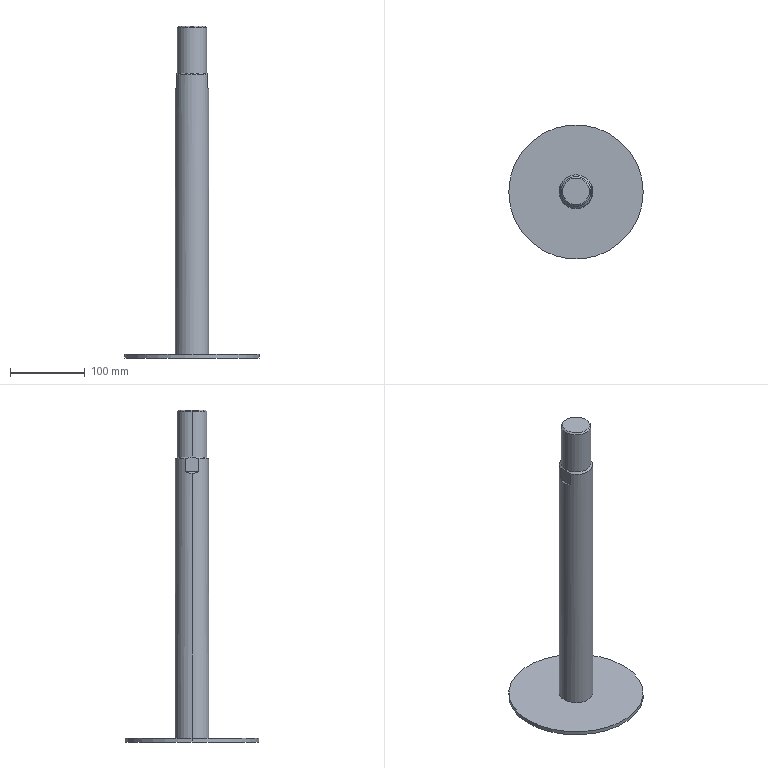Part | STEP file | CDS1FN180-250-A54Z_CS1-Rod | 1 solid | 17 faces | box 180 x 180 x 445 mm | volume 804374 mm3 | plane 7 | cylinder 6 | cone 4 | commonest cylinder face diameters 40 x2 45 x2 180 x2